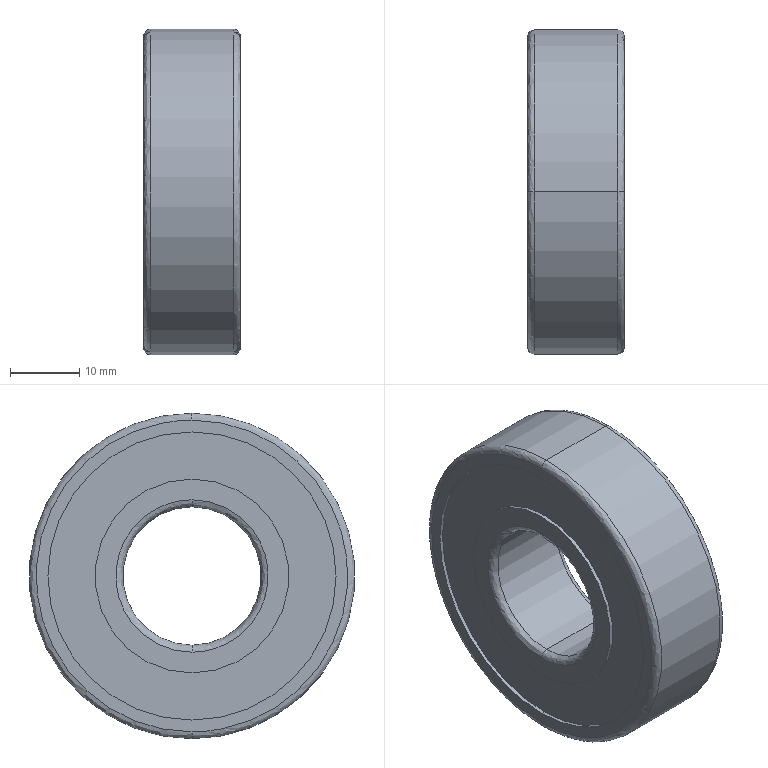Part | STEP file | 1.6米B6204ZZ | 1 solid | 26 faces | box 14 x 47 x 47 mm | volume 19015 mm3 | cylinder 12 | spline 8 | plane 6 | commonest cylinder face diameters 28 x4 41.6 x4 20 x2 47 x2
STEP:
#1=CARTESIAN_POINT('',(14.,0.,-22.5));
#2=VERTEX_POINT('',#1);
#3=CARTESIAN_POINT('',(14.,0.,22.5));
#4=VERTEX_POINT('',#3);
#5=CARTESIAN_POINT('',(14.,0.,-22.5));
#6=CARTESIAN_POINT('',(14.,-45.,-22.5));
#7=CARTESIAN_POINT('',(14.,-45.,22.5));
#8=CARTESIAN_POINT('',(14.,0.,22.5));
#9=(BOUNDED_CURVE()B_SPLINE_CURVE(3,(#5,#6,#7,#8),.UNSPECIFIED.,.F.,.F.)B_SPLINE_CURVE_WITH_KNOTS((4,4),(0.,0.5),.UNSPECIFIED.)CURVE()GEOMETRIC_REPRESENTATION_ITEM()RATIONAL_B_SPLINE_CURVE((1.,0.3333,0.3333,1.))REPRESENTATION_ITEM(''));
#10=EDGE_CURVE('',#2,#4,#9,.T.);
#11=ORIENTED_EDGE('',*,*,#10,.T.);
#12=CARTESIAN_POINT('',(13.,0.,23.5));
#13=VERTEX_POINT('',#12);
#14=CARTESIAN_POINT('',(13.,0.,22.5));
#15=DIRECTION('',(0.,-1.,0.));
#16=DIRECTION('',(0.,0.,1.));
#17=AXIS2_PLACEMENT_3D('',#14,#15,#16);
#18=CIRCLE('',#17,1.);
#19=EDGE_CURVE('',#4,#13,#18,.T.);
#20=ORIENTED_EDGE('',*,*,#19,.T.);
#21=CARTESIAN_POINT('',(13.,0.,-23.5));
#22=VERTEX_POINT('',#21);
#23=CARTESIAN_POINT('',(13.,0.,0.));
#24=DIRECTION('',(-1.,0.,0.));
#25=DIRECTION('',(0.,0.,1.));
#26=AXIS2_PLACEMENT_3D('',#23,#24,#25);
#27=CIRCLE('',#26,23.5);
#28=EDGE_CURVE('',#22,#13,#27,.T.);
#29=ORIENTED_EDGE('',*,*,#28,.F.);
#30=CARTESIAN_POINT('',(13.,0.,-22.5));
#31=DIRECTION('',(0.,1.,0.));
#32=DIRECTION('',(0.,0.,-1.));
#33=AXIS2_PLACEMENT_3D('',#30,#31,#32);
#34=CIRCLE('',#33,1.);
#35=EDGE_CURVE('',#2,#22,#34,.T.);
#36=ORIENTED_EDGE('',*,*,#35,.F.);
#37=EDGE_LOOP('',(#11,#20,#29,#36));
#38=FACE_OUTER_BOUND('',#37,.T.);
#39=CARTESIAN_POINT('',(14.,0.,22.5));
#40=CARTESIAN_POINT('',(14.,-45.,22.5));
#41=CARTESIAN_POINT('',(14.,-45.,-22.5));
#42=CARTESIAN_POINT('',(14.,0.,-22.5));
#43=CARTESIAN_POINT('',(14.,0.,23.086));
#44=CARTESIAN_POINT('',(14.,-46.172,23.086));
#45=CARTESIAN_POINT('',(14.,-46.172,-23.086));
#46=CARTESIAN_POINT('',(14.,0.,-23.086));
#47=CARTESIAN_POINT('',(13.586,0.,23.5));
#48=CARTESIAN_POINT('',(13.586,-47.,23.5));
#49=CARTESIAN_POINT('',(13.586,-47.,-23.5));
#50=CARTESIAN_POINT('',(13.586,0.,-23.5));
#51=CARTESIAN_POINT('',(13.,0.,23.5));
#52=CARTESIAN_POINT('',(13.,-47.,23.5));
#53=CARTESIAN_POINT('',(13.,-47.,-23.5));
#54=CARTESIAN_POINT('',(13.,0.,-23.5));
#55=(BOUNDED_SURFACE()B_SPLINE_SURFACE(3,3,((#39,#40,#41,#42),(#43,#44,#45,#46),(#47,#48,#49,#50),(#51,#52,#53,#54)),.UNSPECIFIED.,.F.,.F.,.F.)B_SPLINE_SURFACE_WITH_KNOTS((4,4),(4,4),(0.,1.),(0.,1.),.UNSPECIFIED.)GEOMETRIC_REPRESENTATION_ITEM()RATIONAL_B_SPLINE_SURFACE(((1.,0.3333,0.3333,1.),(0.8047,0.2682,0.2682,0.8047),(0.8047,0.2682,0.2682,0.8047),(1.,0.3333,0.3333,1.)))REPRESENTATION_ITEM('')SURFACE());
#56=ADVANCED_FACE('',(#38),#55,.T.);
#57=CARTESIAN_POINT('',(1.,0.,23.5));
#58=VERTEX_POINT('',#57);
#59=CARTESIAN_POINT('',(1.,0.,-23.5));
#60=VERTEX_POINT('',#59);
#61=CARTESIAN_POINT('',(1.,0.,0.));
#62=DIRECTION('',(1.,0.,0.));
#63=DIRECTION('',(0.,0.,1.));
#64=AXIS2_PLACEMENT_3D('',#61,#62,#63);
#65=CIRCLE('',#64,23.5);
#66=EDGE_CURVE('',#58,#60,#65,.T.);
#67=ORIENTED_EDGE('',*,*,#66,.F.);
#68=CARTESIAN_POINT('',(0.,0.,22.5));
#69=VERTEX_POINT('',#68);
#70=CARTESIAN_POINT('',(1.,0.,22.5));
#71=DIRECTION('',(0.,-1.,0.));
#72=DIRECTION('',(0.,0.,1.));
#73=AXIS2_PLACEMENT_3D('',#70,#71,#72);
#74=CIRCLE('',#73,1.);
#75=EDGE_CURVE('',#58,#69,#74,.T.);
#76=ORIENTED_EDGE('',*,*,#75,.T.);
#77=CARTESIAN_POINT('',(0.,0.,-22.5));
#78=VERTEX_POINT('',#77);
#79=CARTESIAN_POINT('',(0.,0.,22.5));
#80=CARTESIAN_POINT('',(0.,-45.,22.5));
#81=CARTESIAN_POINT('',(0.,-45.,-22.5));
#82=CARTESIAN_POINT('',(0.,0.,-22.5));
#83=(BOUNDED_CURVE()B_SPLINE_CURVE(3,(#79,#80,#81,#82),.UNSPECIFIED.,.F.,.F.)B_SPLINE_CURVE_WITH_KNOTS((4,4),(0.5,1.),.UNSPECIFIED.)CURVE()GEOMETRIC_REPRESENTATION_ITEM()RATIONAL_B_SPLINE_CURVE((1.,0.3333,0.3333,1.))REPRESENTATION_ITEM(''));
#84=EDGE_CURVE('',#69,#78,#83,.T.);
#85=ORIENTED_EDGE('',*,*,#84,.T.);
#86=CARTESIAN_POINT('',(1.,0.,-22.5));
#87=DIRECTION('',(0.,1.,0.));
#88=DIRECTION('',(0.,0.,-1.));
#89=AXIS2_PLACEMENT_3D('',#86,#87,#88);
#90=CIRCLE('',#89,1.);
#91=EDGE_CURVE('',#60,#78,#90,.T.);
#92=ORIENTED_EDGE('',*,*,#91,.F.);
#93=EDGE_LOOP('',(#67,#76,#85,#92));
#94=FACE_OUTER_BOUND('',#93,.T.);
#95=CARTESIAN_POINT('',(1.,0.,23.5));
#96=CARTESIAN_POINT('',(1.,-47.,23.5));
#97=CARTESIAN_POINT('',(1.,-47.,-23.5));
#98=CARTESIAN_POINT('',(1.,0.,-23.5));
#99=CARTESIAN_POINT('',(0.4142,0.,23.5));
#100=CARTESIAN_POINT('',(0.4142,-47.,23.5));
#101=CARTESIAN_POINT('',(0.4142,-47.,-23.5));
#102=CARTESIAN_POINT('',(0.4142,0.,-23.5));
#103=CARTESIAN_POINT('',(0.,0.,23.086));
#104=CARTESIAN_POINT('',(0.,-46.172,23.086));
#105=CARTESIAN_POINT('',(0.,-46.172,-23.086));
#106=CARTESIAN_POINT('',(0.,0.,-23.086));
#107=CARTESIAN_POINT('',(0.,0.,22.5));
#108=CARTESIAN_POINT('',(0.,-45.,22.5));
#109=CARTESIAN_POINT('',(0.,-45.,-22.5));
#110=CARTESIAN_POINT('',(0.,0.,-22.5));
#111=(BOUNDED_SURFACE()B_SPLINE_SURFACE(3,3,((#95,#96,#97,#98),(#99,#100,#101,#102),(#103,#104,#105,#106),(#107,#108,#109,#110)),.UNSPECIFIED.,.F.,.F.,.F.)B_SPLINE_SURFACE_WITH_KNOTS((4,4),(4,4),(0.,1.),(0.,1.),.UNSPECIFIED.)GEOMETRIC_REPRESENTATION_ITEM()RATIONAL_B_SPLINE_SURFACE(((1.,0.3333,0.3333,1.),(0.8047,0.2682,0.2682,0.8047),(0.8047,0.2682,0.2682,0.8047),(1.,0.3333,0.3333,1.)))REPRESENTATION_ITEM('')SURFACE());
#112=ADVANCED_FACE('',(#94),#111,.T.);
#113=CARTESIAN_POINT('',(13.,0.,-10.));
#114=VERTEX_POINT('',#113);
#115=CARTESIAN_POINT('',(13.,0.,10.));
#116=VERTEX_POINT('',#115);
#117=CARTESIAN_POINT('',(13.,0.,0.));
#118=DIRECTION('',(-1.,0.,0.));
#119=DIRECTION('',(0.,0.,-1.));
#120=AXIS2_PLACEMENT_3D('',#117,#118,#119);
#121=CIRCLE('',#120,10.);
#122=EDGE_CURVE('',#114,#116,#121,.T.);
#123=ORIENTED_EDGE('',*,*,#122,.T.);
#124=CARTESIAN_POINT('',(14.,0.,11.));
#125=VERTEX_POINT('',#124);
#126=CARTESIAN_POINT('',(13.,0.,11.));
#127=DIRECTION('',(0.,-1.,0.));
#128=DIRECTION('',(0.,0.,1.));
#129=AXIS2_PLACEMENT_3D('',#126,#127,#128);
#130=CIRCLE('',#129,1.);
#131=EDGE_CURVE('',#116,#125,#130,.T.);
#132=ORIENTED_EDGE('',*,*,#131,.T.);
#133=CARTESIAN_POINT('',(14.,0.,-11.));
#134=VERTEX_POINT('',#133);
#135=CARTESIAN_POINT('',(14.,0.,-11.));
#136=CARTESIAN_POINT('',(14.,-0.3363,-11.));
#137=CARTESIAN_POINT('',(14.,-0.8388,-10.977));
#138=CARTESIAN_POINT('',(14.,-1.421,-10.91));
#139=CARTESIAN_POINT('',(14.,-1.712,-10.867));
#140=CARTESIAN_POINT('',(14.,-1.857,-10.842));
#141=CARTESIAN_POINT('',(14.,-1.919,-10.831));
#142=CARTESIAN_POINT('',(14.,-1.96,-10.824));
#143=CARTESIAN_POINT('',(14.,-1.98,-10.82));
#144=CARTESIAN_POINT('',(14.,-2.352,-10.751));
#145=CARTESIAN_POINT('',(14.,-2.871,-10.629));
#146=CARTESIAN_POINT('',(14.,-3.464,-10.443));
#147=CARTESIAN_POINT('',(14.,-3.758,-10.339));
#148=CARTESIAN_POINT('',(14.,-3.883,-10.292));
#149=CARTESIAN_POINT('',(14.,-3.966,-10.26));
#150=CARTESIAN_POINT('',(14.,-4.006,-10.245));
#151=CARTESIAN_POINT('',(14.,-4.395,-10.091));
#152=CARTESIAN_POINT('',(14.,-4.9,-9.861));
#153=CARTESIAN_POINT('',(14.,-5.467,-9.548));
#154=CARTESIAN_POINT('',(14.,-5.705,-9.405));
#155=CARTESIAN_POINT('',(14.,-5.863,-9.308));
#156=CARTESIAN_POINT('',(14.,-5.94,-9.259));
#157=CARTESIAN_POINT('',(14.,-6.655,-8.792));
#158=CARTESIAN_POINT('',(14.,-7.241,-8.315));
#159=CARTESIAN_POINT('',(14.,-8.047,-7.51));
#160=CARTESIAN_POINT('',(14.,-8.426,-7.089));
#161=CARTESIAN_POINT('',(14.,-8.83,-6.565));
#162=CARTESIAN_POINT('',(14.,-8.994,-6.333));
#163=CARTESIAN_POINT('',(14.,-9.102,-6.178));
#164=CARTESIAN_POINT('',(14.,-9.156,-6.097));
#165=CARTESIAN_POINT('',(14.,-9.41,-5.708));
#166=CARTESIAN_POINT('',(14.,-9.69,-5.229));
#167=CARTESIAN_POINT('',(14.,-9.974,-4.647));
#168=CARTESIAN_POINT('',(14.,-10.104,-4.35));
#169=CARTESIAN_POINT('',(14.,-10.158,-4.221));
#170=CARTESIAN_POINT('',(14.,-10.193,-4.135));
#171=CARTESIAN_POINT('',(14.,-10.211,-4.09));
#172=CARTESIAN_POINT('',(14.,-10.359,-3.718));
#173=CARTESIAN_POINT('',(14.,-10.531,-3.213));
#174=CARTESIAN_POINT('',(14.,-10.688,-2.612));
#175=CARTESIAN_POINT('',(14.,-10.756,-2.308));
#176=CARTESIAN_POINT('',(14.,-10.787,-2.155));
#177=CARTESIAN_POINT('',(14.,-10.8,-2.089));
#178=CARTESIAN_POINT('',(14.,-10.808,-2.045));
#179=CARTESIAN_POINT('',(14.,-10.813,-2.022));
#180=CARTESIAN_POINT('',(14.,-10.939,-1.34));
#181=CARTESIAN_POINT('',(14.,-11.,-0.6725));
#182=CARTESIAN_POINT('',(14.,-11.,0.3362));
#183=CARTESIAN_POINT('',(14.,-10.977,0.8386));
#184=CARTESIAN_POINT('',(14.,-10.91,1.421));
#185=CARTESIAN_POINT('',(14.,-10.867,1.712));
#186=CARTESIAN_POINT('',(14.,-10.842,1.857));
#187=CARTESIAN_POINT('',(14.,-10.831,1.919));
#188=CARTESIAN_POINT('',(14.,-10.824,1.96));
#189=CARTESIAN_POINT('',(14.,-10.82,1.98));
#190=CARTESIAN_POINT('',(14.,-10.751,2.352));
#191=CARTESIAN_POINT('',(14.,-10.629,2.871));
#192=CARTESIAN_POINT('',(14.,-10.443,3.464));
#193=CARTESIAN_POINT('',(14.,-10.339,3.758));
#194=CARTESIAN_POINT('',(14.,-10.292,3.883));
#195=CARTESIAN_POINT('',(14.,-10.26,3.966));
#196=CARTESIAN_POINT('',(14.,-10.245,4.006));
#197=CARTESIAN_POINT('',(14.,-10.091,4.395));
#198=CARTESIAN_POINT('',(14.,-9.861,4.9));
#199=CARTESIAN_POINT('',(14.,-9.548,5.467));
#200=CARTESIAN_POINT('',(14.,-9.405,5.705));
#201=CARTESIAN_POINT('',(14.,-9.308,5.863));
#202=CARTESIAN_POINT('',(14.,-9.259,5.94));
#203=CARTESIAN_POINT('',(14.,-8.792,6.655));
#204=CARTESIAN_POINT('',(14.,-8.315,7.241));
#205=CARTESIAN_POINT('',(14.,-7.51,8.047));
#206=CARTESIAN_POINT('',(14.,-7.089,8.426));
#207=CARTESIAN_POINT('',(14.,-6.565,8.83));
#208=CARTESIAN_POINT('',(14.,-6.333,8.994));
#209=CARTESIAN_POINT('',(14.,-6.178,9.102));
#210=CARTESIAN_POINT('',(14.,-6.097,9.156));
#211=CARTESIAN_POINT('',(14.,-5.708,9.41));
#212=CARTESIAN_POINT('',(14.,-5.229,9.69));
#213=CARTESIAN_POINT('',(14.,-4.647,9.974));
#214=CARTESIAN_POINT('',(14.,-4.35,10.104));
#215=CARTESIAN_POINT('',(14.,-4.221,10.158));
#216=CARTESIAN_POINT('',(14.,-4.135,10.193));
#217=CARTESIAN_POINT('',(14.,-4.09,10.211));
#218=CARTESIAN_POINT('',(14.,-3.718,10.359));
#219=CARTESIAN_POINT('',(14.,-3.213,10.531));
#220=CARTESIAN_POINT('',(14.,-2.612,10.688));
#221=CARTESIAN_POINT('',(14.,-2.308,10.756));
#222=CARTESIAN_POINT('',(14.,-2.155,10.787));
#223=CARTESIAN_POINT('',(14.,-2.089,10.8));
#224=CARTESIAN_POINT('',(14.,-2.045,10.808));
#225=CARTESIAN_POINT('',(14.,-2.022,10.813));
#226=CARTESIAN_POINT('',(14.,-1.34,10.939));
#227=CARTESIAN_POINT('',(14.,-0.6725,11.));
#228=CARTESIAN_POINT('',(14.,0.,11.));
#229=B_SPLINE_CURVE_WITH_KNOTS('',3,(#135,#136,#137,#138,#139,#140,#141,#142,#143,#144,#145,#146,#147,#148,#149,#150,#151,#152,#153,#154,#155,#156,#157,#158,#159,#160,#161,#162,#163,#164,#165,#166,#167,#168,#169,#170,#171,#172,#173,#174,#175,#176,#177,#178,#179,#180,#181,#182,#183,#184,#185,#186,#187,#188,#189,#190,#191,#192,#193,#194,#195,#196,#197,#198,#199,#200,#201,#202,#203,#204,#205,#206,#207,#208,#209,#210,#211,#212,#213,#214,#215,#216,#217,#218,#219,#220,#221,#222,#223,#224,#225,#226,#227,#228),.UNSPECIFIED.,.F.,.F.,(4,1,1,1,1,2,2,1,1,1,2,2,1,1,2,2,2,1,1,2,2,1,1,1,2,2,1,1,1,1,2,2,2,1,1,1,1,2,2,1,1,1,2,2,1,1,2,2,2,1,1,2,2,1,1,1,2,2,1,1,1,1,2,2,4),(0.,0.01563,0.02344,0.02734,0.0293,0.03027,0.03125,0.04688,0.05469,0.05859,0.06055,0.0625,0.07813,0.08594,0.08984,0.09375,0.125,0.1406,0.1484,0.1523,0.1562,0.1719,0.1797,0.1836,0.1855,0.1875,0.2031,0.2109,0.2148,0.2168,0.2178,0.2187,0.25,0.2656,0.2734,0.2773,0.2793,0.2803,0.2812,0.2969,0.3047,0.3086,0.3105,0.3125,0.3281,0.3359,0.3398,0.3438,0.375,0.3906,0.3984,0.4023,0.4063,0.4219,0.4297,0.4336,0.4355,0.4375,0.4531,0.4609,0.4648,0.4668,0.4678,0.4688,0.5),.UNSPECIFIED.);
#230=EDGE_CURVE('',#134,#125,#229,.T.);
#231=ORIENTED_EDGE('',*,*,#230,.F.);
#232=CARTESIAN_POINT('',(13.,0.,-11.));
#233=DIRECTION('',(0.,1.,0.));
#234=DIRECTION('',(0.,0.,-1.));
#235=AXIS2_PLACEMENT_3D('',#232,#233,#234);
#236=CIRCLE('',#235,1.);
#237=EDGE_CURVE('',#114,#134,#236,.T.);
#238=ORIENTED_EDGE('',*,*,#237,.F.);
#239=EDGE_LOOP('',(#123,#132,#231,#238));
#240=FACE_OUTER_BOUND('',#239,.T.);
#241=CARTESIAN_POINT('',(13.,0.,10.));
#242=CARTESIAN_POINT('',(13.,-20.,10.));
#243=CARTESIAN_POINT('',(13.,-20.,-10.));
#244=CARTESIAN_POINT('',(13.,0.,-10.));
#245=CARTESIAN_POINT('',(13.586,0.,10.));
#246=CARTESIAN_POINT('',(13.586,-20.,10.));
#247=CARTESIAN_POINT('',(13.586,-20.,-10.));
#248=CARTESIAN_POINT('',(13.586,0.,-10.));
#249=CARTESIAN_POINT('',(14.,0.,10.414));
#250=CARTESIAN_POINT('',(14.,-20.828,10.414));
#251=CARTESIAN_POINT('',(14.,-20.828,-10.414));
#252=CARTESIAN_POINT('',(14.,0.,-10.414));
#253=CARTESIAN_POINT('',(14.,0.,11.));
#254=CARTESIAN_POINT('',(14.,-22.,11.));
#255=CARTESIAN_POINT('',(14.,-22.,-11.));
#256=CARTESIAN_POINT('',(14.,0.,-11.));
#257=(BOUNDED_SURFACE()B_SPLINE_SURFACE(3,3,((#241,#242,#243,#244),(#245,#246,#247,#248),(#249,#250,#251,#252),(#253,#254,#255,#256)),.UNSPECIFIED.,.F.,.F.,.T.)B_SPLINE_SURFACE_WITH_KNOTS((4,4),(4,4),(0.,1.),(0.,1.),.UNSPECIFIED.)GEOMETRIC_REPRESENTATION_ITEM()RATIONAL_B_SPLINE_SURFACE(((1.,0.3333,0.3333,1.),(0.8047,0.2682,0.2682,0.8047),(0.8047,0.2682,0.2682,0.8047),(1.,0.3333,0.3333,1.)))REPRESENTATION_ITEM('')SURFACE());
#258=ADVANCED_FACE('',(#240),#257,.T.);
#259=CARTESIAN_POINT('',(0.,0.,11.));
#260=VERTEX_POINT('',#259);
#261=CARTESIAN_POINT('',(0.,0.,-11.));
#262=VERTEX_POINT('',#261);
#263=CARTESIAN_POINT('',(0.,0.,11.));
#264=CARTESIAN_POINT('',(0.,-0.3362,11.));
#265=CARTESIAN_POINT('',(0.,-0.8386,10.977));
#266=CARTESIAN_POINT('',(0.,-1.421,10.91));
#267=CARTESIAN_POINT('',(0.,-1.712,10.867));
#268=CARTESIAN_POINT('',(0.,-1.857,10.842));
#269=CARTESIAN_POINT('',(0.,-1.919,10.831));
#270=CARTESIAN_POINT('',(0.,-1.96,10.824));
#271=CARTESIAN_POINT('',(0.,-1.98,10.82));
#272=CARTESIAN_POINT('',(0.,-2.352,10.751));
#273=CARTESIAN_POINT('',(0.,-2.871,10.629));
#274=CARTESIAN_POINT('',(0.,-3.464,10.443));
#275=CARTESIAN_POINT('',(0.,-3.758,10.339));
#276=CARTESIAN_POINT('',(0.,-3.883,10.292));
#277=CARTESIAN_POINT('',(0.,-3.966,10.26));
#278=CARTESIAN_POINT('',(0.,-4.006,10.245));
#279=CARTESIAN_POINT('',(0.,-4.395,10.091));
#280=CARTESIAN_POINT('',(0.,-4.9,9.861));
#281=CARTESIAN_POINT('',(0.,-5.467,9.548));
#282=CARTESIAN_POINT('',(0.,-5.705,9.405));
#283=CARTESIAN_POINT('',(0.,-5.863,9.308));
#284=CARTESIAN_POINT('',(0.,-5.94,9.259));
#285=CARTESIAN_POINT('',(0.,-6.655,8.792));
#286=CARTESIAN_POINT('',(0.,-7.241,8.315));
#287=CARTESIAN_POINT('',(0.,-8.047,7.51));
#288=CARTESIAN_POINT('',(0.,-8.426,7.089));
#289=CARTESIAN_POINT('',(0.,-8.83,6.565));
#290=CARTESIAN_POINT('',(0.,-8.994,6.333));
#291=CARTESIAN_POINT('',(0.,-9.102,6.178));
#292=CARTESIAN_POINT('',(0.,-9.156,6.097));
#293=CARTESIAN_POINT('',(0.,-9.41,5.708));
#294=CARTESIAN_POINT('',(0.,-9.69,5.229));
#295=CARTESIAN_POINT('',(0.,-9.974,4.647));
#296=CARTESIAN_POINT('',(0.,-10.104,4.35));
#297=CARTESIAN_POINT('',(0.,-10.158,4.221));
#298=CARTESIAN_POINT('',(0.,-10.193,4.135));
#299=CARTESIAN_POINT('',(0.,-10.211,4.09));
#300=CARTESIAN_POINT('',(0.,-10.359,3.718));
#301=CARTESIAN_POINT('',(0.,-10.531,3.213));
#302=CARTESIAN_POINT('',(0.,-10.688,2.612));
#303=CARTESIAN_POINT('',(0.,-10.756,2.308));
#304=CARTESIAN_POINT('',(0.,-10.787,2.155));
#305=CARTESIAN_POINT('',(0.,-10.8,2.089));
#306=CARTESIAN_POINT('',(0.,-10.808,2.045));
#307=CARTESIAN_POINT('',(0.,-10.813,2.022));
#308=CARTESIAN_POINT('',(0.,-10.939,1.34));
#309=CARTESIAN_POINT('',(0.,-11.,0.6725));
#310=CARTESIAN_POINT('',(0.,-11.,-0.3362));
#311=CARTESIAN_POINT('',(0.,-10.977,-0.8386));
#312=CARTESIAN_POINT('',(0.,-10.91,-1.421));
#313=CARTESIAN_POINT('',(0.,-10.867,-1.712));
#314=CARTESIAN_POINT('',(0.,-10.842,-1.857));
#315=CARTESIAN_POINT('',(0.,-10.831,-1.919));
#316=CARTESIAN_POINT('',(0.,-10.824,-1.96));
#317=CARTESIAN_POINT('',(0.,-10.82,-1.98));
#318=CARTESIAN_POINT('',(0.,-10.751,-2.352));
#319=CARTESIAN_POINT('',(0.,-10.629,-2.871));
#320=CARTESIAN_POINT('',(0.,-10.443,-3.464));
#321=CARTESIAN_POINT('',(0.,-10.339,-3.758));
#322=CARTESIAN_POINT('',(0.,-10.292,-3.883));
#323=CARTESIAN_POINT('',(0.,-10.26,-3.966));
#324=CARTESIAN_POINT('',(0.,-10.245,-4.006));
#325=CARTESIAN_POINT('',(0.,-10.091,-4.395));
#326=CARTESIAN_POINT('',(0.,-9.861,-4.9));
#327=CARTESIAN_POINT('',(0.,-9.548,-5.467));
#328=CARTESIAN_POINT('',(0.,-9.405,-5.705));
#329=CARTESIAN_POINT('',(0.,-9.308,-5.863));
#330=CARTESIAN_POINT('',(0.,-9.259,-5.94));
#331=CARTESIAN_POINT('',(0.,-8.792,-6.655));
#332=CARTESIAN_POINT('',(0.,-8.315,-7.241));
#333=CARTESIAN_POINT('',(0.,-7.51,-8.047));
#334=CARTESIAN_POINT('',(0.,-7.089,-8.426));
#335=CARTESIAN_POINT('',(0.,-6.565,-8.83));
#336=CARTESIAN_POINT('',(0.,-6.333,-8.994));
#337=CARTESIAN_POINT('',(0.,-6.178,-9.102));
#338=CARTESIAN_POINT('',(0.,-6.097,-9.156));
#339=CARTESIAN_POINT('',(0.,-5.708,-9.41));
#340=CARTESIAN_POINT('',(0.,-5.229,-9.69));
#341=CARTESIAN_POINT('',(0.,-4.647,-9.974));
#342=CARTESIAN_POINT('',(0.,-4.35,-10.104));
#343=CARTESIAN_POINT('',(0.,-4.221,-10.158));
#344=CARTESIAN_POINT('',(0.,-4.135,-10.193));
#345=CARTESIAN_POINT('',(0.,-4.09,-10.211));
#346=CARTESIAN_POINT('',(0.,-3.718,-10.359));
#347=CARTESIAN_POINT('',(0.,-3.213,-10.531));
#348=CARTESIAN_POINT('',(0.,-2.612,-10.688));
#349=CARTESIAN_POINT('',(0.,-2.308,-10.756));
#350=CARTESIAN_POINT('',(0.,-2.155,-10.787));
#351=CARTESIAN_POINT('',(0.,-2.089,-10.8));
#352=CARTESIAN_POINT('',(0.,-2.045,-10.808));
#353=CARTESIAN_POINT('',(0.,-2.022,-10.813));
#354=CARTESIAN_POINT('',(0.,-1.34,-10.939));
#355=CARTESIAN_POINT('',(0.,-0.673,-11.));
#356=CARTESIAN_POINT('',(0.,0.,-11.));
#357=B_SPLINE_CURVE_WITH_KNOTS('',3,(#263,#264,#265,#266,#267,#268,#269,#270,#271,#272,#273,#274,#275,#276,#277,#278,#279,#280,#281,#282,#283,#284,#285,#286,#287,#288,#289,#290,#291,#292,#293,#294,#295,#296,#297,#298,#299,#300,#301,#302,#303,#304,#305,#306,#307,#308,#309,#310,#311,#312,#313,#314,#315,#316,#317,#318,#319,#320,#321,#322,#323,#324,#325,#326,#327,#328,#329,#330,#331,#332,#333,#334,#335,#336,#337,#338,#339,#340,#341,#342,#343,#344,#345,#346,#347,#348,#349,#350,#351,#352,#353,#354,#355,#356),.UNSPECIFIED.,.F.,.F.,(4,1,1,1,1,2,2,1,1,1,2,2,1,1,2,2,2,1,1,2,2,1,1,1,2,2,1,1,1,1,2,2,2,1,1,1,1,2,2,1,1,1,2,2,1,1,2,2,2,1,1,2,2,1,1,1,2,2,1,1,1,1,2,2,4),(0.5,0.5156,0.5234,0.5273,0.5293,0.5303,0.5313,0.5469,0.5547,0.5586,0.5605,0.5625,0.5781,0.5859,0.5898,0.5938,0.625,0.6406,0.6484,0.6523,0.6562,0.6719,0.6797,0.6836,0.6855,0.6875,0.7031,0.7109,0.7148,0.7168,0.7178,0.7187,0.75,0.7656,0.7734,0.7773,0.7793,0.7803,0.7812,0.7969,0.8047,0.8086,0.8105,0.8125,0.8281,0.8359,0.8398,0.8437,0.875,0.8906,0.8984,0.9023,0.9062,0.9219,0.9297,0.9336,0.9355,0.9375,0.9531,0.9609,0.9648,0.9668,0.9678,0.9687,1.),.UNSPECIFIED.);
#358=EDGE_CURVE('',#260,#262,#357,.T.);
#359=ORIENTED_EDGE('',*,*,#358,.F.);
#360=CARTESIAN_POINT('',(1.,0.,10.));
#361=VERTEX_POINT('',#360);
#362=CARTESIAN_POINT('',(1.,0.,11.));
#363=DIRECTION('',(0.,-1.,0.));
#364=DIRECTION('',(0.,0.,1.));
#365=AXIS2_PLACEMENT_3D('',#362,#363,#364);
#366=CIRCLE('',#365,1.);
#367=EDGE_CURVE('',#260,#361,#366,.T.);
#368=ORIENTED_EDGE('',*,*,#367,.T.);
#369=CARTESIAN_POINT('',(1.,0.,-10.));
#370=VERTEX_POINT('',#369);
#371=CARTESIAN_POINT('',(1.,0.,0.));
#372=DIRECTION('',(1.,0.,0.));
#373=DIRECTION('',(0.,0.,-1.));
#374=AXIS2_PLACEMENT_3D('',#371,#372,#373);
#375=CIRCLE('',#374,10.);
#376=EDGE_CURVE('',#361,#370,#375,.T.);
#377=ORIENTED_EDGE('',*,*,#376,.T.);
#378=CARTESIAN_POINT('',(1.,0.,-11.));
#379=DIRECTION('',(0.,1.,0.));
#380=DIRECTION('',(0.,0.,-1.));
#381=AXIS2_PLACEMENT_3D('',#378,#379,#380);
#382=CIRCLE('',#381,1.);
#383=EDGE_CURVE('',#262,#370,#382,.T.);
#384=ORIENTED_EDGE('',*,*,#383,.F.);
#385=EDGE_LOOP('',(#359,#368,#377,#384));
#386=FACE_OUTER_BOUND('',#385,.T.);
#387=CARTESIAN_POINT('',(0.,0.,11.));
#388=CARTESIAN_POINT('',(0.,-22.,11.));
#389=CARTESIAN_POINT('',(0.,-22.,-11.));
#390=CARTESIAN_POINT('',(0.,0.,-11.));
#391=CARTESIAN_POINT('',(0.,0.,10.414));
#392=CARTESIAN_POINT('',(0.,-20.828,10.414));
#393=CARTESIAN_POINT('',(0.,-20.828,-10.414));
#394=CARTESIAN_POINT('',(0.,0.,-10.414));
#395=CARTESIAN_POINT('',(0.4142,0.,10.));
#396=CARTESIAN_POINT('',(0.4142,-20.,10.));
#397=CARTESIAN_POINT('',(0.4142,-20.,-10.));
#398=CARTESIAN_POINT('',(0.4142,0.,-10.));
#399=CARTESIAN_POINT('',(1.,0.,10.));
#400=CARTESIAN_POINT('',(1.,-20.,10.));
#401=CARTESIAN_POINT('',(1.,-20.,-10.));
#402=CARTESIAN_POINT('',(1.,0.,-10.));
#403=(BOUNDED_SURFACE()B_SPLINE_SURFACE(3,3,((#387,#388,#389,#390),(#391,#392,#393,#394),(#395,#396,#397,#398),(#399,#400,#401,#402)),.UNSPECIFIED.,.F.,.F.,.F.)B_SPLINE_SURFACE_WITH_KNOTS((4,4),(4,4),(0.,1.),(0.,1.),.UNSPECIFIED.)GEOMETRIC_REPRESENTATION_ITEM()RATIONAL_B_SPLINE_SURFACE(((1.,0.3333,0.3333,1.),(0.8047,0.2682,0.2682,0.8047),(0.8047,0.2682,0.2682,0.8047),(1.,0.3333,0.3333,1.)))REPRESENTATION_ITEM('')SURFACE());
#404=ADVANCED_FACE('',(#386),#403,.T.);
#405=CARTESIAN_POINT('',(13.,0.,0.));
#406=DIRECTION('',(-1.,0.,0.));
#407=DIRECTION('',(0.,0.,1.));
#408=AXIS2_PLACEMENT_3D('',#405,#406,#407);
#409=CIRCLE('',#408,23.5);
#410=EDGE_CURVE('',#13,#22,#409,.T.);
#411=ORIENTED_EDGE('',*,*,#410,.T.);
#412=CARTESIAN_POINT('',(14.,0.,-23.5));
#413=DIRECTION('',(-1.,0.,0.));
#414=VECTOR('',#413,1000.);
#415=LINE('',#412,#414);
#416=EDGE_CURVE('',#22,#60,#415,.T.);
#417=ORIENTED_EDGE('',*,*,#416,.T.);
#418=CARTESIAN_POINT('',(1.,0.,0.));
#419=DIRECTION('',(1.,0.,0.));
#420=DIRECTION('',(0.,0.,1.));
#421=AXIS2_PLACEMENT_3D('',#418,#419,#420);
#422=CIRCLE('',#421,23.5);
#423=EDGE_CURVE('',#60,#58,#422,.T.);
#424=ORIENTED_EDGE('',*,*,#423,.T.);
#425=CARTESIAN_POINT('',(14.,0.,23.5));
#426=DIRECTION('',(-1.,0.,0.));
#427=VECTOR('',#426,1000.);
#428=LINE('',#425,#427);
#429=EDGE_CURVE('',#13,#58,#428,.T.);
#430=ORIENTED_EDGE('',*,*,#429,.F.);
#431=EDGE_LOOP('',(#411,#417,#424,#430));
#432=FACE_OUTER_BOUND('',#431,.T.);
#433=CARTESIAN_POINT('',(14.,0.,0.));
#434=DIRECTION('',(-1.,0.,0.));
#435=DIRECTION('',(0.,0.,1.));
#436=AXIS2_PLACEMENT_3D('',#433,#434,#435);
#437=CYLINDRICAL_SURFACE('',#436,23.5);
#438=ADVANCED_FACE('',(#432),#437,.T.);
#439=CARTESIAN_POINT('',(14.,0.,-20.8));
#440=VERTEX_POINT('',#439);
#441=CARTESIAN_POINT('',(14.,0.,20.8));
#442=VERTEX_POINT('',#441);
#443=CARTESIAN_POINT('',(14.,0.,0.));
#444=DIRECTION('',(-1.,0.,0.));
#445=DIRECTION('',(0.,0.,1.));
#446=AXIS2_PLACEMENT_3D('',#443,#444,#445);
#447=CIRCLE('',#446,20.8);
#448=EDGE_CURVE('',#440,#442,#447,.T.);
#449=ORIENTED_EDGE('',*,*,#448,.F.);
#450=CARTESIAN_POINT('',(13.47,0.,-20.8));
#451=VERTEX_POINT('',#450);
#452=CARTESIAN_POINT('',(14.,0.,-20.8));
#453=DIRECTION('',(-1.,0.,0.));
#454=VECTOR('',#453,1000.);
#455=LINE('',#452,#454);
#456=EDGE_CURVE('',#440,#451,#455,.T.);
#457=ORIENTED_EDGE('',*,*,#456,.T.);
#458=CARTESIAN_POINT('',(13.47,0.,20.8));
#459=VERTEX_POINT('',#458);
#460=CARTESIAN_POINT('',(13.47,0.,0.));
#461=DIRECTION('',(1.,0.,0.));
#462=DIRECTION('',(0.,0.,1.));
#463=AXIS2_PLACEMENT_3D('',#460,#461,#462);
#464=CIRCLE('',#463,20.8);
#465=EDGE_CURVE('',#459,#451,#464,.T.);
#466=ORIENTED_EDGE('',*,*,#465,.F.);
#467=CARTESIAN_POINT('',(14.,0.,20.8));
#468=DIRECTION('',(-1.,0.,0.));
#469=VECTOR('',#468,1000.);
#470=LINE('',#467,#469);
#471=EDGE_CURVE('',#442,#459,#470,.T.);
#472=ORIENTED_EDGE('',*,*,#471,.F.);
#473=EDGE_LOOP('',(#449,#457,#466,#472));
#474=FACE_OUTER_BOUND('',#473,.T.);
#475=CARTESIAN_POINT('',(14.,0.,0.));
#476=DIRECTION('',(-1.,0.,0.));
#477=DIRECTION('',(0.,0.,1.));
#478=AXIS2_PLACEMENT_3D('',#475,#476,#477);
#479=CYLINDRICAL_SURFACE('',#478,20.8);
#480=ADVANCED_FACE('',(#474),#479,.F.);
#481=CARTESIAN_POINT('',(0.53,0.,-20.8));
#482=VERTEX_POINT('',#481);
#483=CARTESIAN_POINT('',(0.53,0.,20.8));
#484=VERTEX_POINT('',#483);
#485=CARTESIAN_POINT('',(0.53,0.,0.));
#486=DIRECTION('',(-1.,0.,0.));
#487=DIRECTION('',(0.,0.,1.));
#488=AXIS2_PLACEMENT_3D('',#485,#486,#487);
#489=CIRCLE('',#488,20.8);
#490=EDGE_CURVE('',#482,#484,#489,.T.);
#491=ORIENTED_EDGE('',*,*,#490,.F.);
#492=CARTESIAN_POINT('',(0.,0.,-20.8));
#493=VERTEX_POINT('',#492);
#494=CARTESIAN_POINT('',(14.,0.,-20.8));
#495=DIRECTION('',(-1.,0.,0.));
#496=VECTOR('',#495,1000.);
#497=LINE('',#494,#496);
#498=EDGE_CURVE('',#482,#493,#497,.T.);
#499=ORIENTED_EDGE('',*,*,#498,.T.);
#500=CARTESIAN_POINT('',(0.,0.,20.8));
#501=VERTEX_POINT('',#500);
#502=CARTESIAN_POINT('',(0.,0.,0.));
#503=DIRECTION('',(1.,0.,0.));
#504=DIRECTION('',(0.,0.,1.));
#505=AXIS2_PLACEMENT_3D('',#502,#503,#504);
#506=CIRCLE('',#505,20.8);
#507=EDGE_CURVE('',#501,#493,#506,.T.);
#508=ORIENTED_EDGE('',*,*,#507,.F.);
#509=CARTESIAN_POINT('',(14.,0.,20.8));
#510=DIRECTION('',(-1.,0.,0.));
#511=VECTOR('',#510,1000.);
#512=LINE('',#509,#511);
#513=EDGE_CURVE('',#484,#501,#512,.T.);
#514=ORIENTED_EDGE('',*,*,#513,.F.);
#515=EDGE_LOOP('',(#491,#499,#508,#514));
#516=FACE_OUTER_BOUND('',#515,.T.);
#517=CARTESIAN_POINT('',(14.,0.,0.));
#518=DIRECTION('',(-1.,0.,0.));
#519=DIRECTION('',(0.,0.,1.));
#520=AXIS2_PLACEMENT_3D('',#517,#518,#519);
#521=CYLINDRICAL_SURFACE('',#520,20.8);
#522=ADVANCED_FACE('',(#516),#521,.F.);
#523=CARTESIAN_POINT('',(14.,0.,14.));
#524=VERTEX_POINT('',#523);
#525=CARTESIAN_POINT('',(14.,0.,-14.));
#526=VERTEX_POINT('',#525);
#527=CARTESIAN_POINT('',(14.,0.,0.));
#528=DIRECTION('',(-1.,0.,0.));
#529=DIRECTION('',(0.,0.,1.));
#530=AXIS2_PLACEMENT_3D('',#527,#528,#529);
#531=CIRCLE('',#530,14.);
#532=EDGE_CURVE('',#524,#526,#531,.T.);
#533=ORIENTED_EDGE('',*,*,#532,.T.);
#534=CARTESIAN_POINT('',(13.47,0.,-14.));
#535=VERTEX_POINT('',#534);
#536=CARTESIAN_POINT('',(14.,0.,-14.));
#537=DIRECTION('',(-1.,0.,0.));
#538=VECTOR('',#537,1000.);
#539=LINE('',#536,#538);
#540=EDGE_CURVE('',#526,#535,#539,.T.);
#541=ORIENTED_EDGE('',*,*,#540,.T.);
#542=CARTESIAN_POINT('',(13.47,0.,14.));
#543=VERTEX_POINT('',#542);
#544=CARTESIAN_POINT('',(13.47,0.,0.));
#545=DIRECTION('',(-1.,0.,0.));
#546=DIRECTION('',(0.,0.,1.));
#547=AXIS2_PLACEMENT_3D('',#544,#545,#546);
#548=CIRCLE('',#547,14.);
#549=EDGE_CURVE('',#543,#535,#548,.T.);
#550=ORIENTED_EDGE('',*,*,#549,.F.);
#551=CARTESIAN_POINT('',(14.,0.,14.));
#552=DIRECTION('',(-1.,0.,0.));
#553=VECTOR('',#552,1000.);
#554=LINE('',#551,#553);
#555=EDGE_CURVE('',#524,#543,#554,.T.);
#556=ORIENTED_EDGE('',*,*,#555,.F.);
#557=EDGE_LOOP('',(#533,#541,#550,#556));
#558=FACE_OUTER_BOUND('',#557,.T.);
#559=CARTESIAN_POINT('',(14.,0.,0.));
#560=DIRECTION('',(-1.,0.,0.));
#561=DIRECTION('',(0.,0.,1.));
#562=AXIS2_PLACEMENT_3D('',#559,#560,#561);
#563=CYLINDRICAL_SURFACE('',#562,14.);
#564=ADVANCED_FACE('',(#558),#563,.T.);
#565=CARTESIAN_POINT('',(0.53,0.,-14.));
#566=VERTEX_POINT('',#565);
#567=CARTESIAN_POINT('',(0.53,0.,14.));
#568=VERTEX_POINT('',#567);
#569=CARTESIAN_POINT('',(0.53,0.,0.));
#570=DIRECTION('',(1.,0.,0.));
#571=DIRECTION('',(0.,0.,1.));
#572=AXIS2_PLACEMENT_3D('',#569,#570,#571);
#573=CIRCLE('',#572,14.);
#574=EDGE_CURVE('',#566,#568,#573,.T.);
#575=ORIENTED_EDGE('',*,*,#574,.F.);
#576=CARTESIAN_POINT('',(0.,0.,-14.));
#577=VERTEX_POINT('',#576);
#578=CARTESIAN_POINT('',(14.,0.,-14.));
#579=DIRECTION('',(-1.,0.,0.));
#580=VECTOR('',#579,1000.);
#581=LINE('',#578,#580);
#582=EDGE_CURVE('',#566,#577,#581,.T.);
#583=ORIENTED_EDGE('',*,*,#582,.T.);
#584=CARTESIAN_POINT('',(0.,0.,14.));
#585=VERTEX_POINT('',#584);
#586=CARTESIAN_POINT('',(0.,0.,0.));
#587=DIRECTION('',(1.,0.,0.));
#588=DIRECTION('',(0.,0.,1.));
#589=AXIS2_PLACEMENT_3D('',#586,#587,#588);
#590=CIRCLE('',#589,14.);
#591=EDGE_CURVE('',#577,#585,#590,.T.);
#592=ORIENTED_EDGE('',*,*,#591,.T.);
#593=CARTESIAN_POINT('',(14.,0.,14.));
#594=DIRECTION('',(-1.,0.,0.));
#595=VECTOR('',#594,1000.);
#596=LINE('',#593,#595);
#597=EDGE_CURVE('',#568,#585,#596,.T.);
#598=ORIENTED_EDGE('',*,*,#597,.F.);
#599=EDGE_LOOP('',(#575,#583,#592,#598));
#600=FACE_OUTER_BOUND('',#599,.T.);
#601=CARTESIAN_POINT('',(14.,0.,0.));
#602=DIRECTION('',(-1.,0.,0.));
#603=DIRECTION('',(0.,0.,1.));
#604=AXIS2_PLACEMENT_3D('',#601,#602,#603);
#605=CYLINDRICAL_SURFACE('',#604,14.);
#606=ADVANCED_FACE('',(#600),#605,.T.);
#607=ORIENTED_EDGE('',*,*,#122,.F.);
#608=CARTESIAN_POINT('',(14.,0.,-10.));
#609=DIRECTION('',(-1.,0.,0.));
#610=VECTOR('',#609,1000.);
#611=LINE('',#608,#610);
#612=EDGE_CURVE('',#114,#370,#611,.T.);
#613=ORIENTED_EDGE('',*,*,#612,.T.);
#614=ORIENTED_EDGE('',*,*,#376,.F.);
#615=CARTESIAN_POINT('',(14.,0.,10.));
#616=DIRECTION('',(-1.,0.,0.));
#617=VECTOR('',#616,1000.);
#618=LINE('',#615,#617);
#619=EDGE_CURVE('',#116,#361,#618,.T.);
#620=ORIENTED_EDGE('',*,*,#619,.F.);
#621=EDGE_LOOP('',(#607,#613,#614,#620));
#622=FACE_OUTER_BOUND('',#621,.T.);
#623=CARTESIAN_POINT('',(14.,0.,0.));
#624=DIRECTION('',(-1.,0.,0.));
#625=DIRECTION('',(0.,0.,1.));
#626=AXIS2_PLACEMENT_3D('',#623,#624,#625);
#627=CYLINDRICAL_SURFACE('',#626,10.);
#628=ADVANCED_FACE('',(#622),#627,.F.);
#629=ORIENTED_EDGE('',*,*,#416,.F.);
#630=ORIENTED_EDGE('',*,*,#28,.T.);
#631=ORIENTED_EDGE('',*,*,#429,.T.);
#632=ORIENTED_EDGE('',*,*,#66,.T.);
#633=EDGE_LOOP('',(#629,#630,#631,#632));
#634=FACE_OUTER_BOUND('',#633,.T.);
#635=CARTESIAN_POINT('',(14.,0.,0.));
#636=DIRECTION('',(-1.,0.,0.));
#637=DIRECTION('',(0.,0.,1.));
#638=AXIS2_PLACEMENT_3D('',#635,#636,#637);
#639=CYLINDRICAL_SURFACE('',#638,23.5);
#640=ADVANCED_FACE('',(#634),#639,.T.);
#641=ORIENTED_EDGE('',*,*,#19,.F.);
#642=CARTESIAN_POINT('',(14.,0.,22.5));
#643=CARTESIAN_POINT('',(14.,45.,22.5));
#644=CARTESIAN_POINT('',(14.,45.,-22.5));
#645=CARTESIAN_POINT('',(14.,0.,-22.5));
#646=(BOUNDED_CURVE()B_SPLINE_CURVE(3,(#642,#643,#644,#645),.UNSPECIFIED.,.F.,.T.)B_SPLINE_CURVE_WITH_KNOTS((4,4),(0.5,1.),.UNSPECIFIED.)CURVE()GEOMETRIC_REPRESENTATION_ITEM()RATIONAL_B_SPLINE_CURVE((1.,0.3333,0.3333,1.))REPRESENTATION_ITEM(''));
#647=EDGE_CURVE('',#4,#2,#646,.T.);
#648=ORIENTED_EDGE('',*,*,#647,.T.);
#649=ORIENTED_EDGE('',*,*,#35,.T.);
#650=ORIENTED_EDGE('',*,*,#410,.F.);
#651=EDGE_LOOP('',(#641,#648,#649,#650));
#652=FACE_OUTER_BOUND('',#651,.T.);
#653=CARTESIAN_POINT('',(14.,0.,-22.5));
#654=CARTESIAN_POINT('',(14.,45.,-22.5));
#655=CARTESIAN_POINT('',(14.,45.,22.5));
#656=CARTESIAN_POINT('',(14.,0.,22.5));
#657=CARTESIAN_POINT('',(14.,0.,-23.086));
#658=CARTESIAN_POINT('',(14.,46.172,-23.086));
#659=CARTESIAN_POINT('',(14.,46.172,23.086));
#660=CARTESIAN_POINT('',(14.,0.,23.086));
#661=CARTESIAN_POINT('',(13.586,0.,-23.5));
#662=CARTESIAN_POINT('',(13.586,47.,-23.5));
#663=CARTESIAN_POINT('',(13.586,47.,23.5));
#664=CARTESIAN_POINT('',(13.586,0.,23.5));
#665=CARTESIAN_POINT('',(13.,0.,-23.5));
#666=CARTESIAN_POINT('',(13.,47.,-23.5));
#667=CARTESIAN_POINT('',(13.,47.,23.5));
#668=CARTESIAN_POINT('',(13.,0.,23.5));
#669=(BOUNDED_SURFACE()B_SPLINE_SURFACE(3,3,((#653,#654,#655,#656),(#657,#658,#659,#660),(#661,#662,#663,#664),(#665,#666,#667,#668)),.UNSPECIFIED.,.F.,.F.,.F.)B_SPLINE_SURFACE_WITH_KNOTS((4,4),(4,4),(0.,1.),(0.,1.),.UNSPECIFIED.)GEOMETRIC_REPRESENTATION_ITEM()RATIONAL_B_SPLINE_SURFACE(((1.,0.3333,0.3333,1.),(0.8047,0.2682,0.2682,0.8047),(0.8047,0.2682,0.2682,0.8047),(1.,0.3333,0.3333,1.)))REPRESENTATION_ITEM('')SURFACE());
#670=ADVANCED_FACE('',(#652),#669,.T.);
#671=ORIENTED_EDGE('',*,*,#75,.F.);
#672=ORIENTED_EDGE('',*,*,#423,.F.);
#673=ORIENTED_EDGE('',*,*,#91,.T.);
#674=CARTESIAN_POINT('',(0.,0.,-22.5));
#675=CARTESIAN_POINT('',(0.,45.,-22.5));
#676=CARTESIAN_POINT('',(0.,45.,22.5));
#677=CARTESIAN_POINT('',(0.,0.,22.5));
#678=(BOUNDED_CURVE()B_SPLINE_CURVE(3,(#674,#675,#676,#677),.UNSPECIFIED.,.F.,.F.)B_SPLINE_CURVE_WITH_KNOTS((4,4),(0.,0.5),.UNSPECIFIED.)CURVE()GEOMETRIC_REPRESENTATION_ITEM()RATIONAL_B_SPLINE_CURVE((1.,0.3333,0.3333,1.))REPRESENTATION_ITEM(''));
#679=EDGE_CURVE('',#78,#69,#678,.T.);
#680=ORIENTED_EDGE('',*,*,#679,.T.);
#681=EDGE_LOOP('',(#671,#672,#673,#680));
#682=FACE_OUTER_BOUND('',#681,.T.);
#683=CARTESIAN_POINT('',(1.,0.,-23.5));
#684=CARTESIAN_POINT('',(1.,47.,-23.5));
#685=CARTESIAN_POINT('',(1.,47.,23.5));
#686=CARTESIAN_POINT('',(1.,0.,23.5));
#687=CARTESIAN_POINT('',(0.4142,0.,-23.5));
#688=CARTESIAN_POINT('',(0.4142,47.,-23.5));
#689=CARTESIAN_POINT('',(0.4142,47.,23.5));
#690=CARTESIAN_POINT('',(0.4142,0.,23.5));
#691=CARTESIAN_POINT('',(0.,0.,-23.086));
#692=CARTESIAN_POINT('',(0.,46.172,-23.086));
#693=CARTESIAN_POINT('',(0.,46.172,23.086));
#694=CARTESIAN_POINT('',(0.,0.,23.086));
#695=CARTESIAN_POINT('',(0.,0.,-22.5));
#696=CARTESIAN_POINT('',(0.,45.,-22.5));
#697=CARTESIAN_POINT('',(0.,45.,22.5));
#698=CARTESIAN_POINT('',(0.,0.,22.5));
#699=(BOUNDED_SURFACE()B_SPLINE_SURFACE(3,3,((#683,#684,#685,#686),(#687,#688,#689,#690),(#691,#692,#693,#694),(#695,#696,#697,#698)),.UNSPECIFIED.,.F.,.F.,.T.)B_SPLINE_SURFACE_WITH_KNOTS((4,4),(4,4),(0.,1.),(0.,1.),.UNSPECIFIED.)GEOMETRIC_REPRESENTATION_ITEM()RATIONAL_B_SPLINE_SURFACE(((1.,0.3333,0.3333,1.),(0.8047,0.2682,0.2682,0.8047),(0.8047,0.2682,0.2682,0.8047),(1.,0.3333,0.3333,1.)))REPRESENTATION_ITEM('')SURFACE());
#700=ADVANCED_FACE('',(#682),#699,.T.);
#701=CARTESIAN_POINT('',(14.,0.,0.));
#702=DIRECTION('',(-1.,0.,0.));
#703=DIRECTION('',(0.,0.,1.));
#704=AXIS2_PLACEMENT_3D('',#701,#702,#703);
#705=CIRCLE('',#704,20.8);
#706=EDGE_CURVE('',#442,#440,#705,.T.);
#707=ORIENTED_EDGE('',*,*,#706,.T.);
#708=ORIENTED_EDGE('',*,*,#448,.T.);
#709=EDGE_LOOP('',(#707,#708));
#710=FACE_BOUND('',#709,.T.);
#711=ORIENTED_EDGE('',*,*,#10,.F.);
#712=ORIENTED_EDGE('',*,*,#647,.F.);
#713=EDGE_LOOP('',(#711,#712));
#714=FACE_OUTER_BOUND('',#713,.T.);
#715=CARTESIAN_POINT('',(14.,20.8,0.));
#716=DIRECTION('',(1.,0.,0.));
#717=DIRECTION('',(0.,0.,-1.));
#718=AXIS2_PLACEMENT_3D('',#715,#716,#717);
#719=PLANE('',#718);
#720=ADVANCED_FACE('',(#710,#714),#719,.T.);
#721=ORIENTED_EDGE('',*,*,#679,.F.);
#722=ORIENTED_EDGE('',*,*,#84,.F.);
#723=EDGE_LOOP('',(#721,#722));
#724=FACE_OUTER_BOUND('',#723,.T.);
#725=ORIENTED_EDGE('',*,*,#507,.T.);
#726=CARTESIAN_POINT('',(0.,0.,0.));
#727=DIRECTION('',(1.,0.,0.));
#728=DIRECTION('',(0.,0.,1.));
#729=AXIS2_PLACEMENT_3D('',#726,#727,#728);
#730=CIRCLE('',#729,20.8);
#731=EDGE_CURVE('',#493,#501,#730,.T.);
#732=ORIENTED_EDGE('',*,*,#731,.T.);
#733=EDGE_LOOP('',(#725,#732));
#734=FACE_BOUND('',#733,.T.);
#735=CARTESIAN_POINT('',(0.,22.5,0.));
#736=DIRECTION('',(-1.,0.,0.));
#737=DIRECTION('',(0.,0.,1.));
#738=AXIS2_PLACEMENT_3D('',#735,#736,#737);
#739=PLANE('',#738);
#740=ADVANCED_FACE('',(#724,#734),#739,.T.);
#741=ORIENTED_EDGE('',*,*,#456,.F.);
#742=ORIENTED_EDGE('',*,*,#706,.F.);
#743=ORIENTED_EDGE('',*,*,#471,.T.);
#744=CARTESIAN_POINT('',(13.47,0.,0.));
#745=DIRECTION('',(1.,0.,0.));
#746=DIRECTION('',(0.,0.,1.));
#747=AXIS2_PLACEMENT_3D('',#744,#745,#746);
#748=CIRCLE('',#747,20.8);
#749=EDGE_CURVE('',#451,#459,#748,.T.);
#750=ORIENTED_EDGE('',*,*,#749,.F.);
#751=EDGE_LOOP('',(#741,#742,#743,#750));
#752=FACE_OUTER_BOUND('',#751,.T.);
#753=CARTESIAN_POINT('',(14.,0.,0.));
#754=DIRECTION('',(-1.,0.,0.));
#755=DIRECTION('',(0.,0.,1.));
#756=AXIS2_PLACEMENT_3D('',#753,#754,#755);
#757=CYLINDRICAL_SURFACE('',#756,20.8);
#758=ADVANCED_FACE('',(#752),#757,.F.);
#759=ORIENTED_EDGE('',*,*,#498,.F.);
#760=CARTESIAN_POINT('',(0.53,0.,0.));
#761=DIRECTION('',(-1.,0.,0.));
#762=DIRECTION('',(0.,0.,1.));
#763=AXIS2_PLACEMENT_3D('',#760,#761,#762);
#764=CIRCLE('',#763,20.8);
#765=EDGE_CURVE('',#484,#482,#764,.T.);
#766=ORIENTED_EDGE('',*,*,#765,.F.);
#767=ORIENTED_EDGE('',*,*,#513,.T.);
#768=ORIENTED_EDGE('',*,*,#731,.F.);
#769=EDGE_LOOP('',(#759,#766,#767,#768));
#770=FACE_OUTER_BOUND('',#769,.T.);
#771=CARTESIAN_POINT('',(14.,0.,0.));
#772=DIRECTION('',(-1.,0.,0.));
#773=DIRECTION('',(0.,0.,1.));
#774=AXIS2_PLACEMENT_3D('',#771,#772,#773);
#775=CYLINDRICAL_SURFACE('',#774,20.8);
#776=ADVANCED_FACE('',(#770),#775,.F.);
#777=ORIENTED_EDGE('',*,*,#549,.T.);
#778=CARTESIAN_POINT('',(13.47,0.,0.));
#779=DIRECTION('',(-1.,0.,0.));
#780=DIRECTION('',(0.,0.,1.));
#781=AXIS2_PLACEMENT_3D('',#778,#779,#780);
#782=CIRCLE('',#781,14.);
#783=EDGE_CURVE('',#535,#543,#782,.T.);
#784=ORIENTED_EDGE('',*,*,#783,.T.);
#785=EDGE_LOOP('',(#777,#784));
#786=FACE_BOUND('',#785,.T.);
#787=ORIENTED_EDGE('',*,*,#465,.T.);
#788=ORIENTED_EDGE('',*,*,#749,.T.);
#789=EDGE_LOOP('',(#787,#788));
#790=FACE_OUTER_BOUND('',#789,.T.);
#791=CARTESIAN_POINT('',(13.47,14.,0.));
#792=DIRECTION('',(1.,0.,0.));
#793=DIRECTION('',(0.,0.,-1.));
#794=AXIS2_PLACEMENT_3D('',#791,#792,#793);
#795=PLANE('',#794);
#796=ADVANCED_FACE('',(#786,#790),#795,.T.);
#797=ORIENTED_EDGE('',*,*,#765,.T.);
#798=ORIENTED_EDGE('',*,*,#490,.T.);
#799=EDGE_LOOP('',(#797,#798));
#800=FACE_OUTER_BOUND('',#799,.T.);
#801=CARTESIAN_POINT('',(0.53,0.,0.));
#802=DIRECTION('',(1.,0.,0.));
#803=DIRECTION('',(0.,0.,1.));
#804=AXIS2_PLACEMENT_3D('',#801,#802,#803);
#805=CIRCLE('',#804,14.);
#806=EDGE_CURVE('',#568,#566,#805,.T.);
#807=ORIENTED_EDGE('',*,*,#806,.T.);
#808=ORIENTED_EDGE('',*,*,#574,.T.);
#809=EDGE_LOOP('',(#807,#808));
#810=FACE_BOUND('',#809,.T.);
#811=CARTESIAN_POINT('',(0.53,20.8,0.));
#812=DIRECTION('',(-1.,0.,0.));
#813=DIRECTION('',(0.,0.,1.));
#814=AXIS2_PLACEMENT_3D('',#811,#812,#813);
#815=PLANE('',#814);
#816=ADVANCED_FACE('',(#800,#810),#815,.T.);
#817=ORIENTED_EDGE('',*,*,#540,.F.);
#818=CARTESIAN_POINT('',(14.,0.,0.));
#819=DIRECTION('',(-1.,0.,0.));
#820=DIRECTION('',(0.,0.,1.));
#821=AXIS2_PLACEMENT_3D('',#818,#819,#820);
#822=CIRCLE('',#821,14.);
#823=EDGE_CURVE('',#526,#524,#822,.T.);
#824=ORIENTED_EDGE('',*,*,#823,.T.);
#825=ORIENTED_EDGE('',*,*,#555,.T.);
#826=ORIENTED_EDGE('',*,*,#783,.F.);
#827=EDGE_LOOP('',(#817,#824,#825,#826));
#828=FACE_OUTER_BOUND('',#827,.T.);
#829=CARTESIAN_POINT('',(14.,0.,0.));
#830=DIRECTION('',(-1.,0.,0.));
#831=DIRECTION('',(0.,0.,1.));
#832=AXIS2_PLACEMENT_3D('',#829,#830,#831);
#833=CYLINDRICAL_SURFACE('',#832,14.);
#834=ADVANCED_FACE('',(#828),#833,.T.);
#835=ORIENTED_EDGE('',*,*,#582,.F.);
#836=ORIENTED_EDGE('',*,*,#806,.F.);
#837=ORIENTED_EDGE('',*,*,#597,.T.);
#838=CARTESIAN_POINT('',(0.,0.,0.));
#839=DIRECTION('',(1.,0.,0.));
#840=DIRECTION('',(0.,0.,1.));
#841=AXIS2_PLACEMENT_3D('',#838,#839,#840);
#842=CIRCLE('',#841,14.);
#843=EDGE_CURVE('',#585,#577,#842,.T.);
#844=ORIENTED_EDGE('',*,*,#843,.T.);
#845=EDGE_LOOP('',(#835,#836,#837,#844));
#846=FACE_OUTER_BOUND('',#845,.T.);
#847=CARTESIAN_POINT('',(14.,0.,0.));
#848=DIRECTION('',(-1.,0.,0.));
#849=DIRECTION('',(0.,0.,1.));
#850=AXIS2_PLACEMENT_3D('',#847,#848,#849);
#851=CYLINDRICAL_SURFACE('',#850,14.);
#852=ADVANCED_FACE('',(#846),#851,.T.);
#853=ORIENTED_EDGE('',*,*,#230,.T.);
#854=CARTESIAN_POINT('',(14.,0.,11.));
#855=CARTESIAN_POINT('',(14.,0.3362,11.));
#856=CARTESIAN_POINT('',(14.,0.8386,10.977));
#857=CARTESIAN_POINT('',(14.,1.421,10.91));
#858=CARTESIAN_POINT('',(14.,1.712,10.867));
#859=CARTESIAN_POINT('',(14.,1.857,10.842));
#860=CARTESIAN_POINT('',(14.,1.919,10.831));
#861=CARTESIAN_POINT('',(14.,1.96,10.824));
#862=CARTESIAN_POINT('',(14.,1.98,10.82));
#863=CARTESIAN_POINT('',(14.,2.352,10.751));
#864=CARTESIAN_POINT('',(14.,2.871,10.629));
#865=CARTESIAN_POINT('',(14.,3.464,10.443));
#866=CARTESIAN_POINT('',(14.,3.758,10.339));
#867=CARTESIAN_POINT('',(14.,3.883,10.292));
#868=CARTESIAN_POINT('',(14.,3.966,10.26));
#869=CARTESIAN_POINT('',(14.,4.006,10.245));
#870=CARTESIAN_POINT('',(14.,4.395,10.091));
#871=CARTESIAN_POINT('',(14.,4.9,9.861));
#872=CARTESIAN_POINT('',(14.,5.467,9.548));
#873=CARTESIAN_POINT('',(14.,5.705,9.405));
#874=CARTESIAN_POINT('',(14.,5.863,9.308));
#875=CARTESIAN_POINT('',(14.,5.94,9.259));
#876=CARTESIAN_POINT('',(14.,6.655,8.792));
#877=CARTESIAN_POINT('',(14.,7.241,8.315));
#878=CARTESIAN_POINT('',(14.,8.047,7.51));
#879=CARTESIAN_POINT('',(14.,8.426,7.089));
#880=CARTESIAN_POINT('',(14.,8.83,6.565));
#881=CARTESIAN_POINT('',(14.,8.994,6.333));
#882=CARTESIAN_POINT('',(14.,9.102,6.178));
#883=CARTESIAN_POINT('',(14.,9.156,6.097));
#884=CARTESIAN_POINT('',(14.,9.41,5.708));
#885=CARTESIAN_POINT('',(14.,9.69,5.229));
#886=CARTESIAN_POINT('',(14.,9.974,4.647));
#887=CARTESIAN_POINT('',(14.,10.104,4.35));
#888=CARTESIAN_POINT('',(14.,10.158,4.221));
#889=CARTESIAN_POINT('',(14.,10.193,4.135));
#890=CARTESIAN_POINT('',(14.,10.211,4.09));
#891=CARTESIAN_POINT('',(14.,10.359,3.718));
#892=CARTESIAN_POINT('',(14.,10.531,3.213));
#893=CARTESIAN_POINT('',(14.,10.688,2.612));
#894=CARTESIAN_POINT('',(14.,10.756,2.308));
#895=CARTESIAN_POINT('',(14.,10.787,2.155));
#896=CARTESIAN_POINT('',(14.,10.8,2.089));
#897=CARTESIAN_POINT('',(14.,10.808,2.045));
#898=CARTESIAN_POINT('',(14.,10.813,2.022));
#899=CARTESIAN_POINT('',(14.,10.939,1.34));
#900=CARTESIAN_POINT('',(14.,11.,0.6725));
#901=CARTESIAN_POINT('',(14.,11.,-0.3362));
#902=CARTESIAN_POINT('',(14.,10.977,-0.8386));
#903=CARTESIAN_POINT('',(14.,10.91,-1.421));
#904=CARTESIAN_POINT('',(14.,10.867,-1.712));
#905=CARTESIAN_POINT('',(14.,10.842,-1.857));
#906=CARTESIAN_POINT('',(14.,10.831,-1.919));
#907=CARTESIAN_POINT('',(14.,10.824,-1.96));
#908=CARTESIAN_POINT('',(14.,10.82,-1.98));
#909=CARTESIAN_POINT('',(14.,10.751,-2.352));
#910=CARTESIAN_POINT('',(14.,10.629,-2.871));
#911=CARTESIAN_POINT('',(14.,10.443,-3.464));
#912=CARTESIAN_POINT('',(14.,10.339,-3.758));
#913=CARTESIAN_POINT('',(14.,10.292,-3.883));
#914=CARTESIAN_POINT('',(14.,10.26,-3.966));
#915=CARTESIAN_POINT('',(14.,10.245,-4.006));
#916=CARTESIAN_POINT('',(14.,10.091,-4.395));
#917=CARTESIAN_POINT('',(14.,9.861,-4.9));
#918=CARTESIAN_POINT('',(14.,9.548,-5.467));
#919=CARTESIAN_POINT('',(14.,9.405,-5.705));
#920=CARTESIAN_POINT('',(14.,9.308,-5.863));
#921=CARTESIAN_POINT('',(14.,9.259,-5.94));
#922=CARTESIAN_POINT('',(14.,8.792,-6.655));
#923=CARTESIAN_POINT('',(14.,8.315,-7.241));
#924=CARTESIAN_POINT('',(14.,7.51,-8.047));
#925=CARTESIAN_POINT('',(14.,7.089,-8.426));
#926=CARTESIAN_POINT('',(14.,6.565,-8.83));
#927=CARTESIAN_POINT('',(14.,6.333,-8.994));
#928=CARTESIAN_POINT('',(14.,6.178,-9.102));
#929=CARTESIAN_POINT('',(14.,6.097,-9.156));
#930=CARTESIAN_POINT('',(14.,5.708,-9.41));
#931=CARTESIAN_POINT('',(14.,5.229,-9.69));
#932=CARTESIAN_POINT('',(14.,4.647,-9.974));
#933=CARTESIAN_POINT('',(14.,4.35,-10.104));
#934=CARTESIAN_POINT('',(14.,4.221,-10.158));
#935=CARTESIAN_POINT('',(14.,4.135,-10.193));
#936=CARTESIAN_POINT('',(14.,4.09,-10.211));
#937=CARTESIAN_POINT('',(14.,3.718,-10.359));
#938=CARTESIAN_POINT('',(14.,3.213,-10.531));
#939=CARTESIAN_POINT('',(14.,2.612,-10.688));
#940=CARTESIAN_POINT('',(14.,2.308,-10.756));
#941=CARTESIAN_POINT('',(14.,2.155,-10.787));
#942=CARTESIAN_POINT('',(14.,2.089,-10.8));
#943=CARTESIAN_POINT('',(14.,2.045,-10.808));
#944=CARTESIAN_POINT('',(14.,2.022,-10.813));
#945=CARTESIAN_POINT('',(14.,1.34,-10.939));
#946=CARTESIAN_POINT('',(14.,0.673,-11.));
#947=CARTESIAN_POINT('',(14.,0.,-11.));
#948=B_SPLINE_CURVE_WITH_KNOTS('',3,(#854,#855,#856,#857,#858,#859,#860,#861,#862,#863,#864,#865,#866,#867,#868,#869,#870,#871,#872,#873,#874,#875,#876,#877,#878,#879,#880,#881,#882,#883,#884,#885,#886,#887,#888,#889,#890,#891,#892,#893,#894,#895,#896,#897,#898,#899,#900,#901,#902,#903,#904,#905,#906,#907,#908,#909,#910,#911,#912,#913,#914,#915,#916,#917,#918,#919,#920,#921,#922,#923,#924,#925,#926,#927,#928,#929,#930,#931,#932,#933,#934,#935,#936,#937,#938,#939,#940,#941,#942,#943,#944,#945,#946,#947),.UNSPECIFIED.,.F.,.F.,(4,1,1,1,1,2,2,1,1,1,2,2,1,1,2,2,2,1,1,2,2,1,1,1,2,2,1,1,1,1,2,2,2,1,1,1,1,2,2,1,1,1,2,2,1,1,2,2,2,1,1,2,2,1,1,1,2,2,1,1,1,1,2,2,4),(0.5,0.5156,0.5234,0.5273,0.5293,0.5303,0.5312,0.5469,0.5547,0.5586,0.5605,0.5625,0.5781,0.5859,0.5898,0.5938,0.625,0.6406,0.6484,0.6523,0.6563,0.6719,0.6797,0.6836,0.6855,0.6875,0.7031,0.7109,0.7148,0.7168,0.7178,0.7188,0.75,0.7656,0.7734,0.7773,0.7793,0.7803,0.7813,0.7969,0.8047,0.8086,0.8105,0.8125,0.8281,0.8359,0.8398,0.8438,0.875,0.8906,0.8984,0.9023,0.9062,0.9219,0.9297,0.9336,0.9355,0.9375,0.9531,0.9609,0.9648,0.9668,0.9678,0.9687,1.),.UNSPECIFIED.);
#949=EDGE_CURVE('',#125,#134,#948,.T.);
#950=ORIENTED_EDGE('',*,*,#949,.T.);
#951=EDGE_LOOP('',(#853,#950));
#952=FACE_BOUND('',#951,.T.);
#953=ORIENTED_EDGE('',*,*,#532,.F.);
#954=ORIENTED_EDGE('',*,*,#823,.F.);
#955=EDGE_LOOP('',(#953,#954));
#956=FACE_OUTER_BOUND('',#955,.T.);
#957=CARTESIAN_POINT('',(14.,11.,0.));
#958=DIRECTION('',(1.,0.,0.));
#959=DIRECTION('',(0.,0.,-1.));
#960=AXIS2_PLACEMENT_3D('',#957,#958,#959);
#961=PLANE('',#960);
#962=ADVANCED_FACE('',(#952,#956),#961,.T.);
#963=ORIENTED_EDGE('',*,*,#843,.F.);
#964=ORIENTED_EDGE('',*,*,#591,.F.);
#965=EDGE_LOOP('',(#963,#964));
#966=FACE_OUTER_BOUND('',#965,.T.);
#967=CARTESIAN_POINT('',(0.,0.,-11.));
#968=CARTESIAN_POINT('',(0.,0.3363,-11.));
#969=CARTESIAN_POINT('',(0.,0.8388,-10.977));
#970=CARTESIAN_POINT('',(0.,1.421,-10.91));
#971=CARTESIAN_POINT('',(0.,1.712,-10.867));
#972=CARTESIAN_POINT('',(0.,1.857,-10.842));
#973=CARTESIAN_POINT('',(0.,1.919,-10.831));
#974=CARTESIAN_POINT('',(0.,1.96,-10.824));
#975=CARTESIAN_POINT('',(0.,1.98,-10.82));
#976=CARTESIAN_POINT('',(0.,2.352,-10.751));
#977=CARTESIAN_POINT('',(0.,2.871,-10.629));
#978=CARTESIAN_POINT('',(0.,3.464,-10.443));
#979=CARTESIAN_POINT('',(0.,3.758,-10.339));
#980=CARTESIAN_POINT('',(0.,3.883,-10.292));
#981=CARTESIAN_POINT('',(0.,3.966,-10.26));
#982=CARTESIAN_POINT('',(0.,4.006,-10.245));
#983=CARTESIAN_POINT('',(0.,4.395,-10.091));
#984=CARTESIAN_POINT('',(0.,4.9,-9.861));
#985=CARTESIAN_POINT('',(0.,5.467,-9.548));
#986=CARTESIAN_POINT('',(0.,5.705,-9.405));
#987=CARTESIAN_POINT('',(0.,5.863,-9.308));
#988=CARTESIAN_POINT('',(0.,5.94,-9.259));
#989=CARTESIAN_POINT('',(0.,6.655,-8.792));
#990=CARTESIAN_POINT('',(0.,7.241,-8.315));
#991=CARTESIAN_POINT('',(0.,8.047,-7.51));
#992=CARTESIAN_POINT('',(0.,8.426,-7.089));
#993=CARTESIAN_POINT('',(0.,8.83,-6.565));
#994=CARTESIAN_POINT('',(0.,8.994,-6.333));
#995=CARTESIAN_POINT('',(0.,9.102,-6.178));
#996=CARTESIAN_POINT('',(0.,9.156,-6.097));
#997=CARTESIAN_POINT('',(0.,9.41,-5.708));
#998=CARTESIAN_POINT('',(0.,9.69,-5.229));
#999=CARTESIAN_POINT('',(0.,9.974,-4.647));
#1000=CARTESIAN_POINT('',(0.,10.104,-4.35));
#1001=CARTESIAN_POINT('',(0.,10.158,-4.221));
#1002=CARTESIAN_POINT('',(0.,10.193,-4.135));
#1003=CARTESIAN_POINT('',(0.,10.211,-4.09));
#1004=CARTESIAN_POINT('',(0.,10.359,-3.718));
#1005=CARTESIAN_POINT('',(0.,10.531,-3.213));
#1006=CARTESIAN_POINT('',(0.,10.688,-2.612));
#1007=CARTESIAN_POINT('',(0.,10.756,-2.308));
#1008=CARTESIAN_POINT('',(0.,10.787,-2.155));
#1009=CARTESIAN_POINT('',(0.,10.8,-2.089));
#1010=CARTESIAN_POINT('',(0.,10.808,-2.045));
#1011=CARTESIAN_POINT('',(0.,10.813,-2.022));
#1012=CARTESIAN_POINT('',(0.,10.939,-1.34));
#1013=CARTESIAN_POINT('',(0.,11.,-0.6725));
#1014=CARTESIAN_POINT('',(0.,11.,0.3362));
#1015=CARTESIAN_POINT('',(0.,10.977,0.8386));
#1016=CARTESIAN_POINT('',(0.,10.91,1.421));
#1017=CARTESIAN_POINT('',(0.,10.867,1.712));
#1018=CARTESIAN_POINT('',(0.,10.842,1.857));
#1019=CARTESIAN_POINT('',(0.,10.831,1.919));
#1020=CARTESIAN_POINT('',(0.,10.824,1.96));
#1021=CARTESIAN_POINT('',(0.,10.82,1.98));
#1022=CARTESIAN_POINT('',(0.,10.751,2.352));
#1023=CARTESIAN_POINT('',(0.,10.629,2.871));
#1024=CARTESIAN_POINT('',(0.,10.443,3.464));
#1025=CARTESIAN_POINT('',(0.,10.339,3.758));
#1026=CARTESIAN_POINT('',(0.,10.292,3.883));
#1027=CARTESIAN_POINT('',(0.,10.26,3.966));
#1028=CARTESIAN_POINT('',(0.,10.245,4.006));
#1029=CARTESIAN_POINT('',(0.,10.091,4.395));
#1030=CARTESIAN_POINT('',(0.,9.861,4.9));
#1031=CARTESIAN_POINT('',(0.,9.548,5.467));
#1032=CARTESIAN_POINT('',(0.,9.405,5.705));
#1033=CARTESIAN_POINT('',(0.,9.308,5.863));
#1034=CARTESIAN_POINT('',(0.,9.259,5.94));
#1035=CARTESIAN_POINT('',(0.,8.792,6.655));
#1036=CARTESIAN_POINT('',(0.,8.315,7.241));
#1037=CARTESIAN_POINT('',(0.,7.51,8.047));
#1038=CARTESIAN_POINT('',(0.,7.089,8.426));
#1039=CARTESIAN_POINT('',(0.,6.565,8.83));
#1040=CARTESIAN_POINT('',(0.,6.333,8.994));
#1041=CARTESIAN_POINT('',(0.,6.178,9.102));
#1042=CARTESIAN_POINT('',(0.,6.097,9.156));
#1043=CARTESIAN_POINT('',(0.,5.708,9.41));
#1044=CARTESIAN_POINT('',(0.,5.229,9.69));
#1045=CARTESIAN_POINT('',(0.,4.647,9.974));
#1046=CARTESIAN_POINT('',(0.,4.35,10.104));
#1047=CARTESIAN_POINT('',(0.,4.221,10.158));
#1048=CARTESIAN_POINT('',(0.,4.135,10.193));
#1049=CARTESIAN_POINT('',(0.,4.09,10.211));
#1050=CARTESIAN_POINT('',(0.,3.718,10.359));
#1051=CARTESIAN_POINT('',(0.,3.213,10.531));
#1052=CARTESIAN_POINT('',(0.,2.612,10.688));
#1053=CARTESIAN_POINT('',(0.,2.308,10.756));
#1054=CARTESIAN_POINT('',(0.,2.155,10.787));
#1055=CARTESIAN_POINT('',(0.,2.089,10.8));
#1056=CARTESIAN_POINT('',(0.,2.045,10.808));
#1057=CARTESIAN_POINT('',(0.,2.022,10.813));
#1058=CARTESIAN_POINT('',(0.,1.34,10.939));
#1059=CARTESIAN_POINT('',(0.,0.6725,11.));
#1060=CARTESIAN_POINT('',(0.,0.,11.));
#1061=B_SPLINE_CURVE_WITH_KNOTS('',3,(#967,#968,#969,#970,#971,#972,#973,#974,#975,#976,#977,#978,#979,#980,#981,#982,#983,#984,#985,#986,#987,#988,#989,#990,#991,#992,#993,#994,#995,#996,#997,#998,#999,#1000,#1001,#1002,#1003,#1004,#1005,#1006,#1007,#1008,#1009,#1010,#1011,#1012,#1013,#1014,#1015,#1016,#1017,#1018,#1019,#1020,#1021,#1022,#1023,#1024,#1025,#1026,#1027,#1028,#1029,#1030,#1031,#1032,#1033,#1034,#1035,#1036,#1037,#1038,#1039,#1040,#1041,#1042,#1043,#1044,#1045,#1046,#1047,#1048,#1049,#1050,#1051,#1052,#1053,#1054,#1055,#1056,#1057,#1058,#1059,#1060),.UNSPECIFIED.,.F.,.F.,(4,1,1,1,1,2,2,1,1,1,2,2,1,1,2,2,2,1,1,2,2,1,1,1,2,2,1,1,1,1,2,2,2,1,1,1,1,2,2,1,1,1,2,2,1,1,2,2,2,1,1,2,2,1,1,1,2,2,1,1,1,1,2,2,4),(0.,0.01562,0.02344,0.02734,0.0293,0.03027,0.03125,0.04687,0.05469,0.05859,0.06055,0.0625,0.07812,0.08594,0.08984,0.09375,0.125,0.1406,0.1484,0.1523,0.1563,0.1719,0.1797,0.1836,0.1855,0.1875,0.2031,0.2109,0.2148,0.2168,0.2178,0.2188,0.25,0.2656,0.2734,0.2773,0.2793,0.2803,0.2812,0.2969,0.3047,0.3086,0.3105,0.3125,0.3281,0.3359,0.3398,0.3437,0.375,0.3906,0.3984,0.4023,0.4062,0.4219,0.4297,0.4336,0.4355,0.4375,0.4531,0.4609,0.4648,0.4668,0.4678,0.4687,0.5),.UNSPECIFIED.);
#1062=EDGE_CURVE('',#262,#260,#1061,.T.);
#1063=ORIENTED_EDGE('',*,*,#1062,.T.);
#1064=ORIENTED_EDGE('',*,*,#358,.T.);
#1065=EDGE_LOOP('',(#1063,#1064));
#1066=FACE_BOUND('',#1065,.T.);
#1067=CARTESIAN_POINT('',(0.,14.,0.));
#1068=DIRECTION('',(-1.,0.,0.));
#1069=DIRECTION('',(0.,0.,1.));
#1070=AXIS2_PLACEMENT_3D('',#1067,#1068,#1069);
#1071=PLANE('',#1070);
#1072=ADVANCED_FACE('',(#966,#1066),#1071,.T.);
#1073=ORIENTED_EDGE('',*,*,#131,.F.);
#1074=CARTESIAN_POINT('',(13.,0.,0.));
#1075=DIRECTION('',(-1.,0.,0.));
#1076=DIRECTION('',(0.,0.,-1.));
#1077=AXIS2_PLACEMENT_3D('',#1074,#1075,#1076);
#1078=CIRCLE('',#1077,10.);
#1079=EDGE_CURVE('',#116,#114,#1078,.T.);
#1080=ORIENTED_EDGE('',*,*,#1079,.T.);
#1081=ORIENTED_EDGE('',*,*,#237,.T.);
#1082=ORIENTED_EDGE('',*,*,#949,.F.);
#1083=EDGE_LOOP('',(#1073,#1080,#1081,#1082));
#1084=FACE_OUTER_BOUND('',#1083,.T.);
#1085=CARTESIAN_POINT('',(13.,0.,-10.));
#1086=CARTESIAN_POINT('',(13.,20.,-10.));
#1087=CARTESIAN_POINT('',(13.,20.,10.));
#1088=CARTESIAN_POINT('',(13.,0.,10.));
#1089=CARTESIAN_POINT('',(13.586,0.,-10.));
#1090=CARTESIAN_POINT('',(13.586,20.,-10.));
#1091=CARTESIAN_POINT('',(13.586,20.,10.));
#1092=CARTESIAN_POINT('',(13.586,0.,10.));
#1093=CARTESIAN_POINT('',(14.,0.,-10.414));
#1094=CARTESIAN_POINT('',(14.,20.828,-10.414));
#1095=CARTESIAN_POINT('',(14.,20.828,10.414));
#1096=CARTESIAN_POINT('',(14.,0.,10.414));
#1097=CARTESIAN_POINT('',(14.,0.,-11.));
#1098=CARTESIAN_POINT('',(14.,22.,-11.));
#1099=CARTESIAN_POINT('',(14.,22.,11.));
#1100=CARTESIAN_POINT('',(14.,0.,11.));
#1101=(BOUNDED_SURFACE()B_SPLINE_SURFACE(3,3,((#1085,#1086,#1087,#1088),(#1089,#1090,#1091,#1092),(#1093,#1094,#1095,#1096),(#1097,#1098,#1099,#1100)),.UNSPECIFIED.,.F.,.F.,.F.)B_SPLINE_SURFACE_WITH_KNOTS((4,4),(4,4),(0.,1.),(0.,1.),.UNSPECIFIED.)GEOMETRIC_REPRESENTATION_ITEM()RATIONAL_B_SPLINE_SURFACE(((1.,0.3333,0.3333,1.),(0.8047,0.2682,0.2682,0.8047),(0.8047,0.2682,0.2682,0.8047),(1.,0.3333,0.3333,1.)))REPRESENTATION_ITEM('')SURFACE());
#1102=ADVANCED_FACE('',(#1084),#1101,.T.);
#1103=ORIENTED_EDGE('',*,*,#367,.F.);
#1104=ORIENTED_EDGE('',*,*,#1062,.F.);
#1105=ORIENTED_EDGE('',*,*,#383,.T.);
#1106=CARTESIAN_POINT('',(1.,0.,0.));
#1107=DIRECTION('',(1.,0.,0.));
#1108=DIRECTION('',(0.,0.,-1.));
#1109=AXIS2_PLACEMENT_3D('',#1106,#1107,#1108);
#1110=CIRCLE('',#1109,10.);
#1111=EDGE_CURVE('',#370,#361,#1110,.T.);
#1112=ORIENTED_EDGE('',*,*,#1111,.T.);
#1113=EDGE_LOOP('',(#1103,#1104,#1105,#1112));
#1114=FACE_OUTER_BOUND('',#1113,.T.);
#1115=CARTESIAN_POINT('',(0.,0.,-11.));
#1116=CARTESIAN_POINT('',(0.,22.,-11.));
#1117=CARTESIAN_POINT('',(0.,22.,11.));
#1118=CARTESIAN_POINT('',(0.,0.,11.));
#1119=CARTESIAN_POINT('',(0.,0.,-10.414));
#1120=CARTESIAN_POINT('',(0.,20.828,-10.414));
#1121=CARTESIAN_POINT('',(0.,20.828,10.414));
#1122=CARTESIAN_POINT('',(0.,0.,10.414));
#1123=CARTESIAN_POINT('',(0.4142,0.,-10.));
#1124=CARTESIAN_POINT('',(0.4142,20.,-10.));
#1125=CARTESIAN_POINT('',(0.4142,20.,10.));
#1126=CARTESIAN_POINT('',(0.4142,0.,10.));
#1127=CARTESIAN_POINT('',(1.,0.,-10.));
#1128=CARTESIAN_POINT('',(1.,20.,-10.));
#1129=CARTESIAN_POINT('',(1.,20.,10.));
#1130=CARTESIAN_POINT('',(1.,0.,10.));
#1131=(BOUNDED_SURFACE()B_SPLINE_SURFACE(3,3,((#1115,#1116,#1117,#1118),(#1119,#1120,#1121,#1122),(#1123,#1124,#1125,#1126),(#1127,#1128,#1129,#1130)),.UNSPECIFIED.,.F.,.F.,.F.)B_SPLINE_SURFACE_WITH_KNOTS((4,4),(4,4),(0.,1.),(0.,1.),.UNSPECIFIED.)GEOMETRIC_REPRESENTATION_ITEM()RATIONAL_B_SPLINE_SURFACE(((1.,0.3333,0.3333,1.),(0.8047,0.2682,0.2682,0.8047),(0.8047,0.2682,0.2682,0.8047),(1.,0.3333,0.3333,1.)))REPRESENTATION_ITEM('')SURFACE());
#1132=ADVANCED_FACE('',(#1114),#1131,.T.);
#1133=ORIENTED_EDGE('',*,*,#612,.F.);
#1134=ORIENTED_EDGE('',*,*,#1079,.F.);
#1135=ORIENTED_EDGE('',*,*,#619,.T.);
#1136=ORIENTED_EDGE('',*,*,#1111,.F.);
#1137=EDGE_LOOP('',(#1133,#1134,#1135,#1136));
#1138=FACE_OUTER_BOUND('',#1137,.T.);
#1139=CARTESIAN_POINT('',(14.,0.,0.));
#1140=DIRECTION('',(-1.,0.,0.));
#1141=DIRECTION('',(0.,0.,1.));
#1142=AXIS2_PLACEMENT_3D('',#1139,#1140,#1141);
#1143=CYLINDRICAL_SURFACE('',#1142,10.);
#1144=ADVANCED_FACE('',(#1138),#1143,.F.);
#1145=CLOSED_SHELL('',(#56,#112,#258,#404,#438,#480,#522,#564,#606,#628,#640,#670,#700,#720,#740,#758,#776,#796,#816,#834,#852,#962,#1072,#1102,#1132,#1144));
#1146=MANIFOLD_SOLID_BREP('',#1145);
#1147=CARTESIAN_POINT('',(0.,0.,0.));
#1148=DIRECTION('',(0.,0.,1.));
#1149=DIRECTION('',(1.,0.,0.));
#1150=AXIS2_PLACEMENT_3D('',#1147,#1148,#1149);
#1151=(LENGTH_UNIT()NAMED_UNIT(*)SI_UNIT(.MILLI.,.METRE.));
#1152=UNCERTAINTY_MEASURE_WITH_UNIT(LENGTH_MEASURE(0.00001),#1151,'','');
#1153=(NAMED_UNIT(*)PLANE_ANGLE_UNIT()SI_UNIT($,.RADIAN.));
#1154=(NAMED_UNIT(*)SI_UNIT($,.STERADIAN.)SOLID_ANGLE_UNIT());
#1155=(GEOMETRIC_REPRESENTATION_CONTEXT(3)GLOBAL_UNCERTAINTY_ASSIGNED_CONTEXT((#1152))GLOBAL_UNIT_ASSIGNED_CONTEXT((#1151,#1153,#1154))REPRESENTATION_CONTEXT('',''));
#1156=ADVANCED_BREP_SHAPE_REPRESENTATION('',(#1146,#1150),#1155);